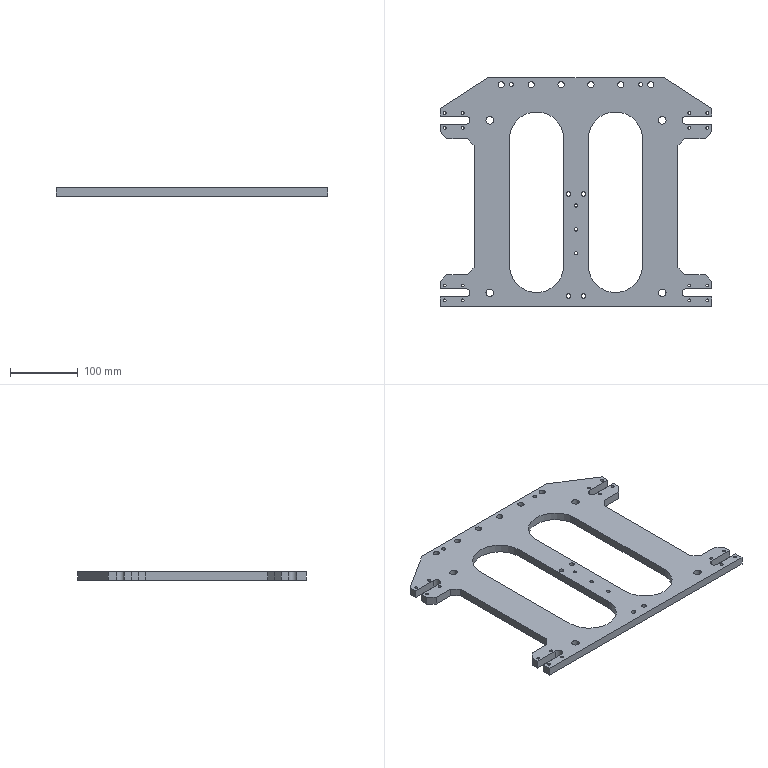NC program | NX | posted with a generic post | part box 400 x 336 x 12 mm
Lines 1 to 1063 of 4851:
N10 G17 G21 G94 G90
(ZLEVEL_PROFILE_COPY_1_1 , TOOL : D10)
N12 T10 M6
N14 G54
N16 G17 G0 G90 X209.776 Y131.22 S2200 M3
N18 G43 Z80. H10
N20 Z2.782
N22 G94 G1 Z-0.218 F2200.
N24 X205.649 Y128.837
N26 G3 X205.149 Y127.971 R1.
N28 G1 X205.15 Y123.041
N30 Y111.5
N32 G2 X200. Y106.35 R5.15
N34 G1 X162.
N36 G3 X161.15 Y105.5 R0.85
N38 X162. Y104.65 R0.85
N40 G1 X200.
N42 G2 X205.15 Y99.5 R5.15
N44 G1 Y89.531
N46 X205.146 Y89.483
N48 X205.09 Y89.281
N50 G2 X203.642 Y84.858 R5.15
N52 G1 X194.375 Y75.592
N54 X194.25 Y75.47
N56 X194.236 Y75.417
N58 X194.182 Y75.407
N60 X194.15 Y75.45
N62 G2 X190. Y73.35 R5.15
N64 G1 X162.133
N66 X155.15 Y66.367
N68 Y-109.367
N70 X162.133 Y-116.35
N72 X189.004
N74 X189.205 Y-116.412
N76 G2 X193.642 Y-117.858 R5.15
N78 G1 X203.642 Y-127.858
N80 G2 X205.15 Y-131.5 R5.15
N82 G1 Y-142.5
N84 G2 X200. Y-147.65 R5.15
N86 G1 X162.
N88 G3 X161.15 Y-148.5 R0.85
N90 X162. Y-149.35 R0.85
N92 G1 X200.
N94 G2 X205.15 Y-154.5 R5.15
N96 G1 Y-164.799
N98 X205.149 Y-172.971
N100 G3 X205.649 Y-173.837 R1.
N102 G1 X209.779 Y-176.222
N104 Z2.782
N106 G0 Z2.564
N108 G1 Z-0.436
N110 X205.649 Y-173.837
N112 G2 X205.149 Y-172.971 R1.
N114 G1 X205.15 Y-164.799
N116 Y-154.5
N118 G3 X200. Y-149.35 R5.15
N120 G1 X162.
N122 G2 X161.15 Y-148.5 R0.85
N124 X162. Y-147.65 R0.85
N126 G1 X200.
N128 G3 X205.15 Y-142.5 R5.15
N130 G1 Y-131.5
N132 G3 X203.642 Y-127.858 R5.15
N134 G1 X193.642 Y-117.858
N136 G3 X189.205 Y-116.412 R5.15
N138 G1 X189.004 Y-116.35
N140 X162.133
N142 X155.15 Y-109.367
N144 Y66.367
N146 X162.133 Y73.35
N148 X190.
N150 G3 X194.15 Y75.45 R5.15
N152 G1 X194.182 Y75.407
N154 X194.236 Y75.417
N156 X194.25 Y75.47
N158 X194.375 Y75.592
N160 X203.642 Y84.858
N162 G3 X205.09 Y89.281 R5.15
N164 G1 X205.146 Y89.483
N166 X205.15 Y89.531
N168 Y99.5
N170 G3 X200. Y104.65 R5.15
N172 G1 X162.
N174 G2 X161.15 Y105.5 R0.85
N176 X162. Y106.35 R0.85
N178 G1 X200.
N180 G3 X205.15 Y111.5 R5.15
N182 G1 Y123.041
N184 X205.149 Y127.971
N186 G2 X205.649 Y128.837 R1.
N188 G1 X209.776 Y131.22
N190 Z2.564
N192 G0 Z2.345
N194 G1 Z-0.655
N196 X205.649 Y128.837
N198 G3 X205.149 Y127.971 R1.
N200 G1 X205.15 Y123.041
N202 Y111.5
N204 G2 X200. Y106.35 R5.15
N206 G1 X162.
N208 G3 X161.15 Y105.5 R0.85
N210 X162. Y104.65 R0.85
N212 G1 X200.
N214 G2 X205.15 Y99.5 R5.15
N216 G1 Y89.531
N218 X205.146 Y89.483
N220 X205.09 Y89.281
N222 G2 X203.642 Y84.858 R5.15
N224 G1 X194.375 Y75.592
N226 X194.25 Y75.47
N228 X194.236 Y75.417
N230 X194.182 Y75.407
N232 X194.15 Y75.45
N234 G2 X190. Y73.35 R5.15
N236 G1 X162.133
N238 X155.15 Y66.367
N240 Y-109.367
N242 X162.133 Y-116.35
N244 X189.004
N246 X189.205 Y-116.412
N248 G2 X193.642 Y-117.858 R5.15
N250 G1 X203.642 Y-127.858
N252 G2 X205.15 Y-131.5 R5.15
N254 G1 Y-142.5
N256 G2 X200. Y-147.65 R5.15
N258 G1 X162.
N260 G3 X161.15 Y-148.5 R0.85
N262 X162. Y-149.35 R0.85
N264 G1 X200.
N266 G2 X205.15 Y-154.5 R5.15
N268 G1 Y-164.799
N270 X205.149 Y-172.971
N272 G3 X205.649 Y-173.837 R1.
N274 G1 X209.779 Y-176.222
N276 Z2.345
N278 G0 Z2.127
N280 G1 Z-0.873
N282 X205.649 Y-173.837
N284 G2 X205.149 Y-172.971 R1.
N286 G1 X205.15 Y-164.799
N288 Y-154.5
N290 G3 X200. Y-149.35 R5.15
N292 G1 X162.
N294 G2 X161.15 Y-148.5 R0.85
N296 X162. Y-147.65 R0.85
N298 G1 X200.
N300 G3 X205.15 Y-142.5 R5.15
N302 G1 Y-131.5
N304 G3 X203.642 Y-127.858 R5.15
N306 G1 X193.642 Y-117.858
N308 G3 X189.205 Y-116.412 R5.15
N310 G1 X189.004 Y-116.35
N312 X162.133
N314 X155.15 Y-109.367
N316 Y66.367
N318 X162.133 Y73.35
N320 X190.
N322 G3 X194.15 Y75.45 R5.15
N324 G1 X194.182 Y75.407
N326 X194.236 Y75.417
N328 X194.25 Y75.47
N330 X194.375 Y75.592
N332 X203.642 Y84.858
N334 G3 X205.09 Y89.281 R5.15
N336 G1 X205.146 Y89.483
N338 X205.15 Y89.531
N340 Y99.5
N342 G3 X200. Y104.65 R5.15
N344 G1 X162.
N346 G2 X161.15 Y105.5 R0.85
N348 X162. Y106.35 R0.85
N350 G1 X200.
N352 G3 X205.15 Y111.5 R5.15
N354 G1 Y123.041
N356 X205.149 Y127.971
N358 G2 X205.649 Y128.837 R1.
N360 G1 X209.776 Y131.22
N362 Z2.127
N364 G0 Z1.909
N366 G1 Z-1.091
N368 X205.649 Y128.837
N370 G3 X205.149 Y127.971 R1.
N372 G1 X205.15 Y123.041
N374 Y111.5
N376 G2 X200. Y106.35 R5.15
N378 G1 X162.
N380 G3 X161.15 Y105.5 R0.85
N382 X162. Y104.65 R0.85
N384 G1 X200.
N386 G2 X205.15 Y99.5 R5.15
N388 G1 Y89.531
N390 X205.146 Y89.483
N392 X205.09 Y89.281
N394 G2 X203.642 Y84.858 R5.15
N396 G1 X194.375 Y75.592
N398 X194.25 Y75.47
N400 X194.236 Y75.417
N402 X194.182 Y75.407
N404 X194.15 Y75.45
N406 G2 X190. Y73.35 R5.15
N408 G1 X162.133
N410 X155.15 Y66.367
N412 Y-109.367
N414 X162.133 Y-116.35
N416 X189.004
N418 X189.205 Y-116.412
N420 G2 X193.642 Y-117.858 R5.15
N422 G1 X203.642 Y-127.858
N424 G2 X205.15 Y-131.5 R5.15
N426 G1 Y-142.5
N428 G2 X200. Y-147.65 R5.15
N430 G1 X162.
N432 G3 X161.15 Y-148.5 R0.85
N434 X162. Y-149.35 R0.85
N436 G1 X200.
N438 G2 X205.15 Y-154.5 R5.15
N440 G1 Y-164.799
N442 X205.149 Y-172.971
N444 G3 X205.649 Y-173.837 R1.
N446 G1 X209.779 Y-176.222
N448 Z1.909
N450 G0 Z1.691
N452 G1 Z-1.309
N454 X205.649 Y-173.837
N456 G2 X205.149 Y-172.971 R1.
N458 G1 X205.15 Y-164.799
N460 Y-154.5
N462 G3 X200. Y-149.35 R5.15
N464 G1 X162.
N466 G2 X161.15 Y-148.5 R0.85
N468 X162. Y-147.65 R0.85
N470 G1 X200.
N472 G3 X205.15 Y-142.5 R5.15
N474 G1 Y-131.5
N476 G3 X203.642 Y-127.858 R5.15
N478 G1 X193.642 Y-117.858
N480 G3 X189.205 Y-116.412 R5.15
N482 G1 X189.004 Y-116.35
N484 X162.133
N486 X155.15 Y-109.367
N488 Y66.367
N490 X162.133 Y73.35
N492 X190.
N494 G3 X194.15 Y75.45 R5.15
N496 G1 X194.182 Y75.407
N498 X194.236 Y75.417
N500 X194.25 Y75.47
N502 X194.375 Y75.592
N504 X203.642 Y84.858
N506 G3 X205.09 Y89.281 R5.15
N508 G1 X205.146 Y89.483
N510 X205.15 Y89.531
N512 Y99.5
N514 G3 X200. Y104.65 R5.15
N516 G1 X162.
N518 G2 X161.15 Y105.5 R0.85
N520 X162. Y106.35 R0.85
N522 G1 X200.
N524 G3 X205.15 Y111.5 R5.15
N526 G1 Y123.041
N528 X205.149 Y127.971
N530 G2 X205.649 Y128.837 R1.
N532 G1 X209.776 Y131.22
N534 Z1.691
N536 G0 Z1.473
N538 G1 Z-1.527
N540 X205.649 Y128.837
N542 G3 X205.149 Y127.971 R1.
N544 G1 X205.15 Y123.041
N546 Y111.5
N548 G2 X200. Y106.35 R5.15
N550 G1 X162.
N552 G3 X161.15 Y105.5 R0.85
N554 X162. Y104.65 R0.85
N556 G1 X200.
N558 G2 X205.15 Y99.5 R5.15
N560 G1 Y89.531
N562 X205.146 Y89.483
N564 X205.09 Y89.281
N566 G2 X203.642 Y84.858 R5.15
N568 G1 X194.375 Y75.592
N570 X194.25 Y75.47
N572 X194.236 Y75.417
N574 X194.182 Y75.407
N576 X194.15 Y75.45
N578 G2 X190. Y73.35 R5.15
N580 G1 X162.133
N582 X155.15 Y66.367
N584 Y-109.367
N586 X162.133 Y-116.35
N588 X189.004
N590 X189.205 Y-116.412
N592 G2 X193.642 Y-117.858 R5.15
N594 G1 X203.642 Y-127.858
N596 G2 X205.15 Y-131.5 R5.15
N598 G1 Y-142.5
N600 G2 X200. Y-147.65 R5.15
N602 G1 X162.
N604 G3 X161.15 Y-148.5 R0.85
N606 X162. Y-149.35 R0.85
N608 G1 X200.
N610 G2 X205.15 Y-154.5 R5.15
N612 G1 Y-164.799
N614 X205.149 Y-172.971
N616 G3 X205.649 Y-173.837 R1.
N618 G1 X209.779 Y-176.222
N620 Z1.473
N622 G0 Z1.255
N624 G1 Z-1.745
N626 X205.649 Y-173.837
N628 G2 X205.149 Y-172.971 R1.
N630 G1 X205.15 Y-164.799
N632 Y-154.5
N634 G3 X200. Y-149.35 R5.15
N636 G1 X162.
N638 G2 X161.15 Y-148.5 R0.85
N640 X162. Y-147.65 R0.85
N642 G1 X200.
N644 G3 X205.15 Y-142.5 R5.15
N646 G1 Y-131.5
N648 G3 X203.642 Y-127.858 R5.15
N650 G1 X193.642 Y-117.858
N652 G3 X189.205 Y-116.412 R5.15
N654 G1 X189.004 Y-116.35
N656 X162.133
N658 X155.15 Y-109.367
N660 Y66.367
N662 X162.133 Y73.35
N664 X190.
N666 G3 X194.15 Y75.45 R5.15
N668 G1 X194.182 Y75.407
N670 X194.236 Y75.417
N672 X194.25 Y75.47
N674 X194.375 Y75.592
N676 X203.642 Y84.858
N678 G3 X205.09 Y89.281 R5.15
N680 G1 X205.146 Y89.483
N682 X205.15 Y89.531
N684 Y99.5
N686 G3 X200. Y104.65 R5.15
N688 G1 X162.
N690 G2 X161.15 Y105.5 R0.85
N692 X162. Y106.35 R0.85
N694 G1 X200.
N696 G3 X205.15 Y111.5 R5.15
N698 G1 Y123.041
N700 X205.149 Y127.971
N702 G2 X205.649 Y128.837 R1.
N704 G1 X209.776 Y131.22
N706 Z1.255
N708 G0 Z1.036
N710 G1 Z-1.964
N712 X205.649 Y128.837
N714 G3 X205.149 Y127.971 R1.
N716 G1 X205.15 Y123.041
N718 Y111.5
N720 G2 X200. Y106.35 R5.15
N722 G1 X162.
N724 G3 X161.15 Y105.5 R0.85
N726 X162. Y104.65 R0.85
N728 G1 X200.
N730 G2 X205.15 Y99.5 R5.15
N732 G1 Y89.531
N734 X205.146 Y89.483
N736 X205.09 Y89.281
N738 G2 X203.642 Y84.858 R5.15
N740 G1 X194.375 Y75.592
N742 X194.25 Y75.47
N744 X194.236 Y75.417
N746 X194.182 Y75.407
N748 X194.15 Y75.45
N750 G2 X190. Y73.35 R5.15
N752 G1 X162.133
N754 X155.15 Y66.367
N756 Y-109.367
N758 X162.133 Y-116.35
N760 X189.004
N762 X189.205 Y-116.412
N764 G2 X193.642 Y-117.858 R5.15
N766 G1 X203.642 Y-127.858
N768 G2 X205.15 Y-131.5 R5.15
N770 G1 Y-142.5
N772 G2 X200. Y-147.65 R5.15
N774 G1 X162.
N776 G3 X161.15 Y-148.5 R0.85
N778 X162. Y-149.35 R0.85
N780 G1 X200.
N782 G2 X205.15 Y-154.5 R5.15
N784 G1 Y-164.799
N786 X205.149 Y-172.971
N788 G3 X205.649 Y-173.837 R1.
N790 G1 X209.779 Y-176.222
N792 Z1.036
N794 G0 Z0.818
N796 G1 Z-2.182
N798 X205.649 Y-173.837
N800 G2 X205.15 Y-172.971 R1.
N802 G1 Y-164.799
N804 Y-154.5
N806 G3 X200. Y-149.35 R5.15
N808 G1 X162.
N810 G2 X161.15 Y-148.5 R0.85
N812 X162. Y-147.65 R0.85
N814 G1 X200.
N816 G3 X205.15 Y-142.5 R5.15
N818 G1 Y-131.5
N820 G3 X203.642 Y-127.858 R5.15
N822 G1 X193.642 Y-117.858
N824 G3 X189.205 Y-116.412 R5.15
N826 G1 X189.004 Y-116.35
N828 X162.133
N830 X155.15 Y-109.367
N832 Y66.367
N834 X162.133 Y73.35
N836 X190.
N838 G3 X194.15 Y75.45 R5.15
N840 G1 X194.182 Y75.407
N842 X194.236 Y75.417
N844 X194.25 Y75.47
N846 X194.375 Y75.592
N848 X203.642 Y84.858
N850 G3 X205.09 Y89.281 R5.15
N852 G1 X205.146 Y89.483
N854 X205.15 Y89.531
N856 Y99.5
N858 G3 X200. Y104.65 R5.15
N860 G1 X162.
N862 G2 X161.15 Y105.5 R0.85
N864 X162. Y106.35 R0.85
N866 G1 X200.
N868 G3 X205.15 Y111.5 R5.15
N870 G1 Y123.041
N872 Y127.971
N874 G2 X205.649 Y128.837 R1.
N876 G1 X209.776 Y131.22
N878 Z0.818
N880 G0 Z0.6
N882 G1 Z-2.4
N884 X205.649 Y128.837
N886 G3 X205.15 Y127.971 R1.
N888 G1 Y123.041
N890 Y111.5
N892 G2 X200. Y106.35 R5.15
N894 G1 X162.
N896 G3 X161.15 Y105.5 R0.85
N898 X162. Y104.65 R0.85
N900 G1 X200.
N902 G2 X205.15 Y99.5 R5.15
N904 G1 Y89.531
N906 X205.146 Y89.483
N908 X205.09 Y89.281
N910 G2 X203.642 Y84.858 R5.15
N912 G1 X194.375 Y75.592
N914 X194.25 Y75.47
N916 X194.236 Y75.417
N918 X194.182 Y75.407
N920 X194.15 Y75.45
N922 G2 X190. Y73.35 R5.15
N924 G1 X162.133
N926 X155.15 Y66.367
N928 Y-109.367
N930 X162.133 Y-116.35
N932 X189.004
N934 X189.205 Y-116.412
N936 G2 X193.642 Y-117.858 R5.15
N938 G1 X203.642 Y-127.858
N940 G2 X205.15 Y-131.5 R5.15
N942 G1 Y-142.5
N944 G2 X200. Y-147.65 R5.15
N946 G1 X162.
N948 G3 X161.15 Y-148.5 R0.85
N950 X162. Y-149.35 R0.85
N952 G1 X200.
N954 G2 X205.15 Y-154.5 R5.15
N956 G1 Y-164.799
N958 Y-172.971
N960 G3 X205.649 Y-173.837 R1.
N962 G1 X209.779 Y-176.222
N964 Z0.6
N966 G0 Z0.382
N968 G1 Z-2.618
N970 X205.649 Y-173.837
N972 G2 X205.15 Y-172.971 R1.
N974 G1 Y-164.799
N976 Y-154.5
N978 G3 X200. Y-149.35 R5.15
N980 G1 X162.
N982 G2 X161.15 Y-148.5 R0.85
N984 X162. Y-147.65 R0.85
N986 G1 X200.
N988 G3 X205.15 Y-142.5 R5.15
N990 G1 Y-131.5
N992 G3 X203.642 Y-127.858 R5.15
N994 G1 X193.642 Y-117.858
N996 G3 X189.205 Y-116.412 R5.15
N998 G1 X189.004 Y-116.35
N1000 X162.133
N1002 X155.15 Y-109.367
N1004 Y66.367
N1006 X162.133 Y73.35
N1008 X190.
N1010 G3 X194.15 Y75.45 R5.15
N1012 G1 X194.182 Y75.407
N1014 X194.236 Y75.417
N1016 X194.25 Y75.47
N1018 X194.375 Y75.592
N1020 X203.642 Y84.858
N1022 G3 X205.09 Y89.281 R5.15
N1024 G1 X205.146 Y89.483
N1026 X205.15 Y89.531
N1028 Y99.5
N1030 G3 X200. Y104.65 R5.15
N1032 G1 X162.
N1034 G2 X161.15 Y105.5 R0.85
N1036 X162. Y106.35 R0.85
N1038 G1 X200.
N1040 G3 X205.15 Y111.5 R5.15
N1042 G1 Y123.041
N1044 Y127.971
N1046 G2 X205.649 Y128.837 R1.
N1048 G1 X209.776 Y131.22
N1050 Z0.382
N1052 G0 Z0.164
N1054 G1 Z-2.836
N1056 X205.649 Y128.837
N1058 G3 X205.15 Y127.971 R1.
N1060 G1 Y123.041
N1062 Y111.5
N1064 G2 X200. Y106.35 R5.15
N1066 G1 X162.
N1068 G3 X161.15 Y105.5 R0.85
N1070 X162. Y104.65 R0.85
N1072 G1 X200.
N1074 G2 X205.15 Y99.5 R5.15
N1076 G1 Y89.531
N1078 X205.146 Y89.483
N1080 X205.09 Y89.281
N1082 G2 X203.642 Y84.858 R5.15
N1084 G1 X194.375 Y75.592
N1086 X194.25 Y75.47
N1088 X194.236 Y75.417
N1090 X194.182 Y75.407
N1092 X194.15 Y75.45
N1094 G2 X190. Y73.35 R5.15
N1096 G1 X162.133
N1098 X155.15 Y66.367
N1100 Y-109.367
N1102 X162.133 Y-116.35
N1104 X189.004
N1106 X189.205 Y-116.412
N1108 G2 X193.642 Y-117.858 R5.15
N1110 G1 X203.642 Y-127.858
N1112 G2 X205.15 Y-131.5 R5.15
N1114 G1 Y-142.5
N1116 G2 X200. Y-147.65 R5.15
N1118 G1 X162.
N1120 G3 X161.15 Y-148.5 R0.85
N1122 X162. Y-149.35 R0.85
N1124 G1 X200.
N1126 G2 X205.15 Y-154.5 R5.15
N1128 G1 Y-164.799
N1130 Y-172.971
N1132 G3 X205.649 Y-173.837 R1.
N1134 G1 X209.779 Y-176.222
N1136 Z0.164
N1138 G0 Z-0.055
N1140 G1 Z-3.055
N1142 X205.649 Y-173.837
N1144 G2 X205.15 Y-172.971 R1.
N1146 G1 Y-164.799
N1148 Y-154.5
N1150 G3 X200. Y-149.35 R5.15
N1152 G1 X162.
N1154 G2 X161.15 Y-148.5 R0.85
N1156 X162. Y-147.65 R0.85
N1158 G1 X200.
N1160 G3 X205.15 Y-142.5 R5.15
N1162 G1 Y-131.5
N1164 G3 X203.642 Y-127.858 R5.15
N1166 G1 X193.642 Y-117.858
N1168 G3 X189.205 Y-116.412 R5.15
N1170 G1 X189.004 Y-116.35
N1172 X162.133
N1174 X155.15 Y-109.367
N1176 Y66.367
N1178 X162.133 Y73.35
N1180 X190.
N1182 G3 X194.15 Y75.45 R5.15
N1184 G1 X194.182 Y75.407
N1186 X194.236 Y75.417
N1188 X194.25 Y75.47
N1190 X194.375 Y75.592
N1192 X203.642 Y84.858
N1194 G3 X205.09 Y89.281 R5.15
N1196 G1 X205.146 Y89.483
N1198 X205.15 Y89.531
N1200 Y99.5
N1202 G3 X200. Y104.65 R5.15
N1204 G1 X162.
N1206 G2 X161.15 Y105.5 R0.85
N1208 X162. Y106.35 R0.85
N1210 G1 X200.
N1212 G3 X205.15 Y111.5 R5.15
N1214 G1 Y123.041
N1216 Y127.971
N1218 G2 X205.649 Y128.837 R1.
N1220 G1 X209.776 Y131.22
N1222 Z-0.055
N1224 G0 Z-0.273
N1226 G1 Z-3.273
N1228 X205.649 Y128.837
N1230 G3 X205.15 Y127.971 R1.
N1232 G1 Y123.041
N1234 Y111.5
N1236 G2 X200. Y106.35 R5.15
N1238 G1 X162.
N1240 G3 X161.15 Y105.5 R0.85
N1242 X162. Y104.65 R0.85
N1244 G1 X200.
N1246 G2 X205.15 Y99.5 R5.15
N1248 G1 Y89.531
N1250 X205.146 Y89.483
N1252 X205.09 Y89.281
N1254 G2 X203.642 Y84.858 R5.15
N1256 G1 X194.375 Y75.592
N1258 X194.25 Y75.47
N1260 X194.236 Y75.417
N1262 X194.182 Y75.407
N1264 X194.15 Y75.45
N1266 G2 X190. Y73.35 R5.15
N1268 G1 X162.133
N1270 X155.15 Y66.367
N1272 Y-109.367
N1274 X162.133 Y-116.35
N1276 X189.004
N1278 X189.205 Y-116.412
N1280 G2 X193.642 Y-117.858 R5.15
N1282 G1 X203.642 Y-127.858
N1284 G2 X205.15 Y-131.5 R5.15
N1286 G1 Y-142.5
N1288 G2 X200. Y-147.65 R5.15
N1290 G1 X162.
N1292 G3 X161.15 Y-148.5 R0.85
N1294 X162. Y-149.35 R0.85
N1296 G1 X200.
N1298 G2 X205.15 Y-154.5 R5.15
N1300 G1 Y-164.799
N1302 Y-172.971
N1304 G3 X205.649 Y-173.837 R1.
N1306 G1 X209.779 Y-176.222
N1308 Z-0.273
N1310 G0 Z-0.491
N1312 G1 Z-3.491
N1314 X205.649 Y-173.837
N1316 G2 X205.15 Y-172.971 R1.
N1318 G1 Y-164.799
N1320 Y-154.5
N1322 G3 X200. Y-149.35 R5.15
N1324 G1 X162.
N1326 G2 X161.15 Y-148.5 R0.85
N1328 X162. Y-147.65 R0.85
N1330 G1 X200.
N1332 G3 X205.15 Y-142.5 R5.15
N1334 G1 Y-131.5
N1336 G3 X203.642 Y-127.858 R5.15
N1338 G1 X193.642 Y-117.858
N1340 G3 X189.205 Y-116.412 R5.15
N1342 G1 X189.004 Y-116.35
N1344 X162.133
N1346 X155.15 Y-109.367
N1348 Y66.367
N1350 X162.133 Y73.35
N1352 X190.
N1354 G3 X194.15 Y75.45 R5.15
N1356 G1 X194.182 Y75.407
N1358 X194.236 Y75.417
N1360 X194.25 Y75.47
N1362 X194.375 Y75.592
N1364 X203.642 Y84.858
N1366 G3 X205.09 Y89.281 R5.15
N1368 G1 X205.146 Y89.483
N1370 X205.15 Y89.531
N1372 Y99.5
N1374 G3 X200. Y104.65 R5.15
N1376 G1 X162.
N1378 G2 X161.15 Y105.5 R0.85
N1380 X162. Y106.35 R0.85
N1382 G1 X200.
N1384 G3 X205.15 Y111.5 R5.15
N1386 G1 Y123.041
N1388 Y127.971
N1390 G2 X205.649 Y128.837 R1.
N1392 G1 X209.776 Y131.22
N1394 Z-0.491
N1396 G0 Z-0.709
N1398 G1 Z-3.709
N1400 X205.649 Y128.837
N1402 G3 X205.15 Y127.971 R1.
N1404 G1 Y123.041
N1406 Y111.5
N1408 G2 X200. Y106.35 R5.15
N1410 G1 X162.
N1412 G3 X161.15 Y105.5 R0.85
N1414 X162. Y104.65 R0.85
N1416 G1 X200.
N1418 G2 X205.15 Y99.5 R5.15
N1420 G1 Y89.531
N1422 X205.146 Y89.483
N1424 X205.09 Y89.281
N1426 G2 X203.642 Y84.858 R5.15
N1428 G1 X194.375 Y75.592
N1430 X194.25 Y75.47
N1432 X194.236 Y75.417
N1434 X194.182 Y75.407
N1436 X194.15 Y75.45
N1438 G2 X190. Y73.35 R5.15
N1440 G1 X162.133
N1442 X155.15 Y66.367
N1444 Y-109.367
N1446 X162.133 Y-116.35
N1448 X189.004
N1450 X189.205 Y-116.412
N1452 G2 X193.642 Y-117.858 R5.15
N1454 G1 X203.642 Y-127.858
N1456 G2 X205.15 Y-131.5 R5.15
N1458 G1 Y-142.5
N1460 G2 X200. Y-147.65 R5.15
N1462 G1 X162.
N1464 G3 X161.15 Y-148.5 R0.85
N1466 X162. Y-149.35 R0.85
N1468 G1 X200.
N1470 G2 X205.15 Y-154.5 R5.15
N1472 G1 Y-164.799
N1474 Y-172.971
N1476 G3 X205.65 Y-173.837 R1.
N1478 G1 X209.779 Y-176.222
N1480 Z-0.709
N1482 G0 Z-0.927
N1484 G1 Z-3.927
N1486 X205.65 Y-173.837
N1488 G2 X205.15 Y-172.971 R1.
N1490 G1 Y-164.799
N1492 Y-154.5
N1494 G3 X200. Y-149.35 R5.15
N1496 G1 X162.
N1498 G2 X161.15 Y-148.5 R0.85
N1500 X162. Y-147.65 R0.85
N1502 G1 X200.
N1504 G3 X205.15 Y-142.5 R5.15
N1506 G1 Y-131.5
N1508 G3 X203.642 Y-127.858 R5.15
N1510 G1 X193.642 Y-117.858
N1512 G3 X189.205 Y-116.412 R5.15
N1514 G1 X189.004 Y-116.35
N1516 X162.133
N1518 X155.15 Y-109.367
N1520 Y66.367
N1522 X162.133 Y73.35
N1524 X190.
N1526 G3 X194.15 Y75.45 R5.15
N1528 G1 X194.182 Y75.407
N1530 X194.236 Y75.417
N1532 X194.25 Y75.47
N1534 X194.375 Y75.592
N1536 X203.642 Y84.858
N1538 G3 X205.09 Y89.281 R5.15
N1540 G1 X205.147 Y89.483
N1542 X205.15 Y89.531
N1544 Y99.5
N1546 G3 X200. Y104.65 R5.15
N1548 G1 X162.
N1550 G2 X161.15 Y105.5 R0.85
N1552 X162. Y106.35 R0.85
N1554 G1 X200.
N1556 G3 X205.15 Y111.5 R5.15
N1558 G1 Y123.041
N1560 Y127.971
N1562 G2 X205.649 Y128.837 R1.
N1564 G1 X209.776 Y131.22
N1566 Z-0.927
N1568 G0 Z-1.145
N1570 G1 Z-4.145
N1572 X205.649 Y128.837
N1574 G3 X205.15 Y127.971 R1.
N1576 G1 Y123.041
N1578 Y111.5
N1580 G2 X200. Y106.35 R5.15
N1582 G1 X162.
N1584 G3 X161.15 Y105.5 R0.85
N1586 X162. Y104.65 R0.85
N1588 G1 X200.
N1590 G2 X205.15 Y99.5 R5.15
N1592 G1 Y89.531
N1594 X205.147 Y89.483
N1596 X205.09 Y89.281
N1598 G2 X203.642 Y84.858 R5.15
N1600 G1 X194.375 Y75.592
N1602 X194.25 Y75.47
N1604 X194.236 Y75.417
N1606 X194.182 Y75.407
N1608 X194.15 Y75.45
N1610 G2 X190. Y73.35 R5.15
N1612 G1 X162.133
N1614 X155.15 Y66.367
N1616 Y-109.367
N1618 X162.133 Y-116.35
N1620 X189.004
N1622 X189.205 Y-116.412
N1624 G2 X193.642 Y-117.858 R5.15
N1626 G1 X203.642 Y-127.858
N1628 G2 X205.15 Y-131.5 R5.15
N1630 G1 Y-142.5
N1632 G2 X200. Y-147.65 R5.15
N1634 G1 X162.
N1636 G3 X161.15 Y-148.5 R0.85
N1638 X162. Y-149.35 R0.85
N1640 G1 X200.
N1642 G2 X205.15 Y-154.5 R5.15
N1644 G1 Y-164.799
N1646 Y-172.971
N1648 G3 X205.65 Y-173.837 R1.
N1650 G1 X209.779 Y-176.222
N1652 Z-1.145
N1654 G0 Z-1.364
N1656 G1 Z-4.364
N1658 X205.65 Y-173.837
N1660 G2 X205.15 Y-172.971 R1.
N1662 G1 Y-164.799
N1664 Y-154.5
N1666 G3 X200. Y-149.35 R5.15
N1668 G1 X162.
N1670 G2 X161.15 Y-148.5 R0.85
N1672 X162. Y-147.65 R0.85
N1674 G1 X200.
N1676 G3 X205.15 Y-142.5 R5.15
N1678 G1 Y-131.5
N1680 G3 X203.642 Y-127.858 R5.15
N1682 G1 X193.642 Y-117.858
N1684 G3 X189.205 Y-116.412 R5.15
N1686 G1 X189.004 Y-116.35
N1688 X162.133
N1690 X155.15 Y-109.367
N1692 Y66.367
N1694 X162.133 Y73.35
N1696 X190.
N1698 G3 X194.15 Y75.45 R5.15
N1700 G1 X194.182 Y75.407
N1702 X194.236 Y75.417
N1704 X194.25 Y75.47
N1706 X194.375 Y75.592
N1708 X203.642 Y84.858
N1710 G3 X205.09 Y89.281 R5.15
N1712 G1 X205.147 Y89.483
N1714 X205.15 Y89.531
N1716 Y99.5
N1718 G3 X200. Y104.65 R5.15
N1720 G1 X162.
N1722 G2 X161.15 Y105.5 R0.85
N1724 X162. Y106.35 R0.85
N1726 G1 X200.
N1728 G3 X205.15 Y111.5 R5.15
N1730 G1 Y123.041
N1732 Y127.971
N1734 G2 X205.649 Y128.837 R1.
N1736 G1 X209.776 Y131.22
N1738 Z-1.364
N1740 G0 Z-1.582
N1742 G1 Z-4.582
N1744 X205.65 Y128.837
N1746 G3 X205.15 Y127.971 R1.
N1748 G1 Y123.041
N1750 Y111.5
N1752 G2 X200. Y106.35 R5.15
N1754 G1 X162.
N1756 G3 X161.15 Y105.5 R0.85
N1758 X162. Y104.65 R0.85
N1760 G1 X200.
N1762 G2 X205.15 Y99.5 R5.15
N1764 G1 Y89.531
N1766 X205.147 Y89.483
N1768 X205.09 Y89.281
N1770 G2 X203.642 Y84.858 R5.15
N1772 G1 X194.375 Y75.592
N1774 X194.25 Y75.47
N1776 X194.236 Y75.417
N1778 X194.182 Y75.407
N1780 X194.15 Y75.45
N1782 G2 X190. Y73.35 R5.15
N1784 G1 X162.133
N1786 X155.15 Y66.367
N1788 Y-109.367
N1790 X162.133 Y-116.35
N1792 X189.004
N1794 X189.205 Y-116.412
N1796 G2 X193.642 Y-117.858 R5.15
N1798 G1 X203.642 Y-127.858
N1800 G2 X205.15 Y-131.5 R5.15
N1802 G1 Y-142.5
N1804 G2 X200. Y-147.65 R5.15
N1806 G1 X162.
N1808 G3 X161.15 Y-148.5 R0.85
N1810 X162. Y-149.35 R0.85
N1812 G1 X200.
N1814 G2 X205.15 Y-154.5 R5.15
N1816 G1 Y-164.799
N1818 Y-172.971
N1820 G3 X205.65 Y-173.837 R1.
N1822 G1 X209.779 Y-176.222
N1824 Z-1.582
N1826 G0 Z-1.8
N1828 G1 Z-4.8
N1830 X205.65 Y-173.837
N1832 G2 X205.15 Y-172.971 R1.
N1834 G1 Y-164.799
N1836 Y-154.5
N1838 G3 X200. Y-149.35 R5.15
N1840 G1 X162.
N1842 G2 X161.15 Y-148.5 R0.85
N1844 X162. Y-147.65 R0.85
N1846 G1 X200.
N1848 G3 X205.15 Y-142.5 R5.15
N1850 G1 Y-131.5
N1852 G3 X203.642 Y-127.858 R5.15
N1854 G1 X193.642 Y-117.858
N1856 G3 X189.205 Y-116.412 R5.15
N1858 G1 X189.004 Y-116.35
N1860 X162.133
N1862 X155.15 Y-109.367
N1864 Y66.367
N1866 X162.133 Y73.35
N1868 X190.
N1870 G3 X194.15 Y75.45 R5.15
N1872 G1 X194.182 Y75.407
N1874 X194.236 Y75.417
N1876 X194.25 Y75.47
N1878 X194.375 Y75.592
N1880 X203.642 Y84.858
N1882 G3 X205.09 Y89.281 R5.15
N1884 G1 X205.147 Y89.483
N1886 X205.15 Y89.531
N1888 Y99.5
N1890 G3 X200. Y104.65 R5.15
N1892 G1 X162.
N1894 G2 X161.15 Y105.5 R0.85
N1896 X162. Y106.35 R0.85
N1898 G1 X200.
N1900 G3 X205.15 Y111.5 R5.15
N1902 G1 Y123.041
N1904 Y127.971
N1906 G2 X205.65 Y128.837 R1.
N1908 G1 X209.776 Y131.22
N1910 Z-1.8
N1912 G0 Z-2.018
N1914 G1 Z-5.018
N1916 X205.65 Y128.837
N1918 G3 X205.15 Y127.971 R1.
N1920 G1 Y123.041
N1922 Y111.5
N1924 G2 X200. Y106.35 R5.15
N1926 G1 X162.
N1928 G3 X161.15 Y105.5 R0.85
N1930 X162. Y104.65 R0.85
N1932 G1 X200.
N1934 G2 X205.15 Y99.5 R5.15
N1936 G1 Y89.531
N1938 X205.147 Y89.483
N1940 X205.09 Y89.281
N1942 G2 X203.642 Y84.858 R5.15
N1944 G1 X194.375 Y75.592
N1946 X194.25 Y75.47
N1948 X194.236 Y75.417
N1950 X194.182 Y75.407
N1952 X194.15 Y75.45
N1954 G2 X190. Y73.35 R5.15
N1956 G1 X162.133
N1958 X155.15 Y66.367
N1960 Y-109.367
N1962 X162.133 Y-116.35
N1964 X189.004
N1966 X189.205 Y-116.412
N1968 G2 X193.642 Y-117.858 R5.15
N1970 G1 X203.642 Y-127.858
N1972 G2 X205.15 Y-131.5 R5.15
N1974 G1 Y-142.5
N1976 G2 X200. Y-147.65 R5.15
N1978 G1 X162.
N1980 G3 X161.15 Y-148.5 R0.85
N1982 X162. Y-149.35 R0.85
N1984 G1 X200.
N1986 G2 X205.15 Y-154.5 R5.15
N1988 G1 Y-164.799
N1990 Y-172.971
N1992 G3 X205.65 Y-173.837 R1.
N1994 G1 X209.779 Y-176.222
N1996 Z-2.018
N1998 G0 Z-2.236
N2000 G1 Z-5.236
N2002 X205.65 Y-173.837
N2004 G2 X205.15 Y-172.971 R1.
N2006 G1 Y-164.799
N2008 Y-154.5
N2010 G3 X200. Y-149.35 R5.15
N2012 G1 X162.
N2014 G2 X161.15 Y-148.5 R0.85
N2016 X162. Y-147.65 R0.85
N2018 G1 X200.
N2020 G3 X205.15 Y-142.5 R5.15
N2022 G1 Y-131.5
N2024 G3 X203.642 Y-127.858 R5.15
N2026 G1 X193.642 Y-117.858
N2028 G3 X189.205 Y-116.412 R5.15
N2030 G1 X189.004 Y-116.35
N2032 X162.133
N2034 X155.15 Y-109.367
N2036 Y66.367
N2038 X162.133 Y73.35
N2040 X190.
N2042 G3 X194.15 Y75.45 R5.15
N2044 G1 X194.182 Y75.407
N2046 X194.236 Y75.417
N2048 X194.25 Y75.47
N2050 X194.375 Y75.592
N2052 X203.642 Y84.858
N2054 G3 X205.09 Y89.281 R5.15
N2056 G1 X205.147 Y89.483
N2058 X205.15 Y89.531
N2060 Y99.5
N2062 G3 X200. Y104.65 R5.15
N2064 G1 X162.
N2066 G2 X161.15 Y105.5 R0.85
N2068 X162. Y106.35 R0.85
N2070 G1 X200.
N2072 G3 X205.15 Y111.5 R5.15
N2074 G1 Y123.041
N2076 Y127.971
N2078 G2 X205.65 Y128.837 R1.
N2080 G1 X209.776 Y131.22
N2082 Z-2.236
N2084 G0 Z-2.455
N2086 G1 Z-5.455
N2088 X205.65 Y128.837
N2090 G3 X205.15 Y127.971 R1.
N2092 G1 Y123.041
N2094 Y111.5
N2096 G2 X200. Y106.35 R5.15
N2098 G1 X162.
N2100 G3 X161.15 Y105.5 R0.85
N2102 X162. Y104.65 R0.85
N2104 G1 X200.
N2106 G2 X205.15 Y99.5 R5.15
N2108 G1 Y89.531
N2110 X205.147 Y89.483
N2112 X205.09 Y89.281
N2114 G2 X203.642 Y84.858 R5.15
N2116 G1 X194.375 Y75.592
N2118 X194.25 Y75.47
N2120 X194.236 Y75.417
N2122 X194.182 Y75.407
N2124 X194.15 Y75.45